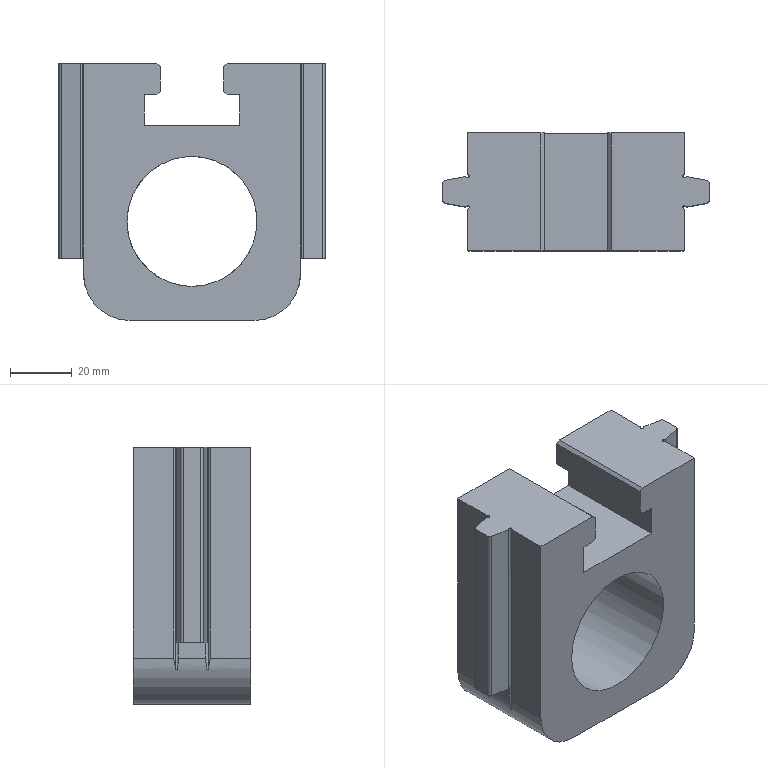Part | STEP file | 冲床-300配套压波_id662_x_t | 1 solid | 58 faces | box 86 x 38 x 83 mm | volume 152874 mm3 | plane 30 | cylinder 22 | cone 6 | commonest cylinder face diameters 1 x12 2 x4 4.2 x3 30 x2 42 x1